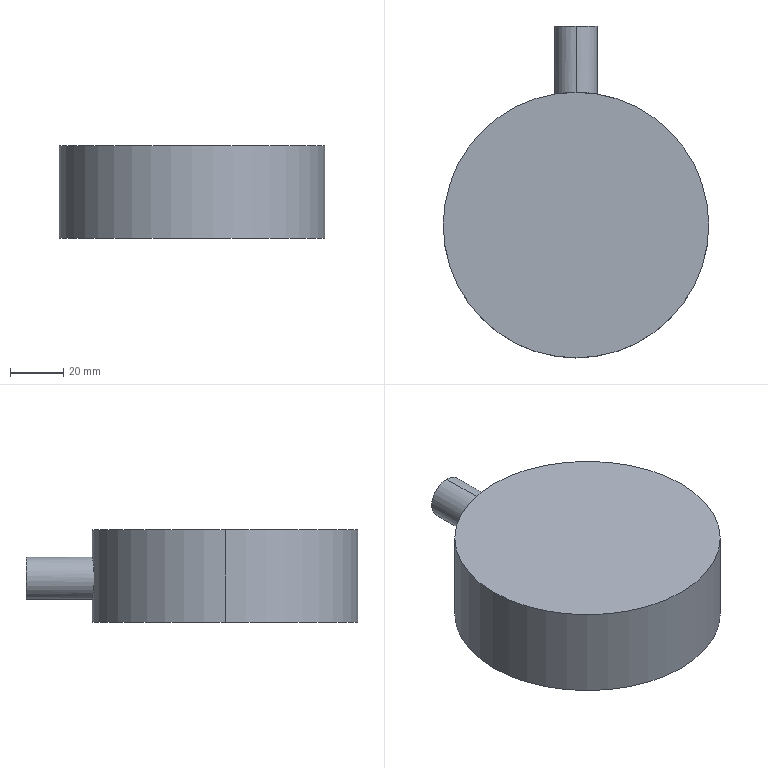Part | SolidWorks | features Extrusion 1, ICE 1 | 1 solid | 7 faces | box 100 x 125 x 35 mm | volume 279948 mm3 | cylinder 4 | plane 3 | commonest cylinder face diameters 16 x2 100 x2
STEP:
#1=CARTESIAN_POINT('',(0.,75.,24.624));
#2=VERTEX_POINT('',#1);
#3=CARTESIAN_POINT('',(0.,75.,8.624));
#4=VERTEX_POINT('',#3);
#5=CARTESIAN_POINT('',(0.,75.,16.624));
#6=DIRECTION('',(0.,1.,0.));
#7=DIRECTION('',(0.,0.,1.));
#8=AXIS2_PLACEMENT_3D('',#5,#6,#7);
#9=CIRCLE('',#8,8.);
#10=EDGE_CURVE('',#2,#4,#9,.T.);
#11=ORIENTED_EDGE('',*,*,#10,.F.);
#12=CARTESIAN_POINT('',(0.,50.,24.624));
#13=VERTEX_POINT('',#12);
#14=CARTESIAN_POINT('',(0.,75.,24.624));
#15=DIRECTION('',(0.,-1.,0.));
#16=VECTOR('',#15,1000.);
#17=LINE('',#14,#16);
#18=EDGE_CURVE('',#2,#13,#17,.T.);
#19=ORIENTED_EDGE('',*,*,#18,.T.);
#20=CARTESIAN_POINT('',(0.,50.,8.624));
#21=VERTEX_POINT('',#20);
#22=CARTESIAN_POINT('',(0.,50.,24.624));
#23=CARTESIAN_POINT('',(0.5224,50.,24.624));
#24=CARTESIAN_POINT('',(1.042,49.992,24.574));
#25=CARTESIAN_POINT('',(1.818,49.968,24.419));
#26=CARTESIAN_POINT('',(2.075,49.958,24.355));
#27=CARTESIAN_POINT('',(2.576,49.934,24.203));
#28=CARTESIAN_POINT('',(3.067,49.908,24.027));
#29=CARTESIAN_POINT('',(3.538,49.875,23.804));
#30=CARTESIAN_POINT('',(4.,49.84,23.557));
#31=CARTESIAN_POINT('',(4.228,49.821,23.421));
#32=CARTESIAN_POINT('',(4.882,49.763,22.984));
#33=CARTESIAN_POINT('',(5.284,49.721,22.653));
#34=CARTESIAN_POINT('',(6.022,49.637,21.916));
#35=CARTESIAN_POINT('',(6.36,49.595,21.505));
#36=CARTESIAN_POINT('',(6.94,49.517,20.638));
#37=CARTESIAN_POINT('',(7.186,49.481,20.179));
#38=CARTESIAN_POINT('',(7.488,49.436,19.452));
#39=CARTESIAN_POINT('',(7.578,49.423,19.203));
#40=CARTESIAN_POINT('',(7.73,49.399,18.701));
#41=CARTESIAN_POINT('',(7.794,49.389,18.447));
#42=CARTESIAN_POINT('',(7.947,49.364,17.68));
#43=CARTESIAN_POINT('',(8.,49.356,17.158));
#44=CARTESIAN_POINT('',(8.,49.356,16.101));
#45=CARTESIAN_POINT('',(7.949,49.364,15.581));
#46=CARTESIAN_POINT('',(7.797,49.388,14.813));
#47=CARTESIAN_POINT('',(7.733,49.398,14.559));
#48=CARTESIAN_POINT('',(7.581,49.422,14.055));
#49=CARTESIAN_POINT('',(7.491,49.436,13.805));
#50=CARTESIAN_POINT('',(7.191,49.481,13.08));
#51=CARTESIAN_POINT('',(6.946,49.516,12.62));
#52=CARTESIAN_POINT('',(6.51,49.575,11.968));
#53=CARTESIAN_POINT('',(6.353,49.595,11.755));
#54=CARTESIAN_POINT('',(6.02,49.637,11.349));
#55=CARTESIAN_POINT('',(5.845,49.658,11.155));
#56=CARTESIAN_POINT('',(5.293,49.72,10.603));
#57=CARTESIAN_POINT('',(4.891,49.762,10.272));
#58=CARTESIAN_POINT('',(4.016,49.84,9.685));
#59=CARTESIAN_POINT('',(3.553,49.876,9.438));
#60=CARTESIAN_POINT('',(2.832,49.92,9.138));
#61=CARTESIAN_POINT('',(2.586,49.934,9.049));
#62=CARTESIAN_POINT('',(2.085,49.957,8.896));
#63=CARTESIAN_POINT('',(1.827,49.967,8.831));
#64=CARTESIAN_POINT('',(1.052,49.992,8.676));
#65=CARTESIAN_POINT('',(0.5294,50.,8.624));
#66=CARTESIAN_POINT('',(0.,50.,8.624));
#67=B_SPLINE_CURVE_WITH_KNOTS('',3,(#22,#23,#24,#25,#26,#27,#28,#29,#30,#31,#32,#33,#34,#35,#36,#37,#38,#39,#40,#41,#42,#43,#44,#45,#46,#47,#48,#49,#50,#51,#52,#53,#54,#55,#56,#57,#58,#59,#60,#61,#62,#63,#64,#65,#66),.UNSPECIFIED.,.F.,.F.,(4,2,2,1,2,2,2,2,2,2,2,2,2,2,2,2,2,2,2,2,2,2,4),(0.02505,0.02662,0.0274,0.02818,0.02897,0.02975,0.03131,0.03288,0.03444,0.03523,0.03601,0.03757,0.03914,0.03992,0.04071,0.04227,0.04305,0.04384,0.0454,0.04697,0.04775,0.04853,0.0501),.UNSPECIFIED.);
#68=EDGE_CURVE('',#13,#21,#67,.T.);
#69=ORIENTED_EDGE('',*,*,#68,.T.);
#70=CARTESIAN_POINT('',(0.,75.,8.624));
#71=DIRECTION('',(0.,-1.,0.));
#72=VECTOR('',#71,1000.);
#73=LINE('',#70,#72);
#74=EDGE_CURVE('',#4,#21,#73,.T.);
#75=ORIENTED_EDGE('',*,*,#74,.F.);
#76=EDGE_LOOP('',(#11,#19,#69,#75));
#77=FACE_OUTER_BOUND('',#76,.T.);
#78=CARTESIAN_POINT('',(0.,75.,16.624));
#79=DIRECTION('',(0.,-1.,0.));
#80=DIRECTION('',(0.,0.,-1.));
#81=AXIS2_PLACEMENT_3D('',#78,#79,#80);
#82=CYLINDRICAL_SURFACE('',#81,8.);
#83=ADVANCED_FACE('',(#77),#82,.T.);
#84=CARTESIAN_POINT('',(0.,50.,8.624));
#85=CARTESIAN_POINT('',(-0.5295,50.,8.624));
#86=CARTESIAN_POINT('',(-1.05,49.992,8.676));
#87=CARTESIAN_POINT('',(-1.818,49.968,8.829));
#88=CARTESIAN_POINT('',(-2.072,49.958,8.893));
#89=CARTESIAN_POINT('',(-2.575,49.934,9.045));
#90=CARTESIAN_POINT('',(-2.824,49.921,9.135));
#91=CARTESIAN_POINT('',(-3.551,49.876,9.436));
#92=CARTESIAN_POINT('',(-4.01,49.841,9.682));
#93=CARTESIAN_POINT('',(-4.662,49.783,10.118));
#94=CARTESIAN_POINT('',(-4.874,49.762,10.275));
#95=CARTESIAN_POINT('',(-5.28,49.721,10.609));
#96=CARTESIAN_POINT('',(-5.474,49.7,10.785));
#97=CARTESIAN_POINT('',(-6.026,49.637,11.337));
#98=CARTESIAN_POINT('',(-6.357,49.595,11.739));
#99=CARTESIAN_POINT('',(-6.796,49.536,12.395));
#100=CARTESIAN_POINT('',(-6.932,49.517,12.622));
#101=CARTESIAN_POINT('',(-7.178,49.482,13.083));
#102=CARTESIAN_POINT('',(-7.401,49.449,13.554));
#103=CARTESIAN_POINT('',(-7.578,49.423,14.046));
#104=CARTESIAN_POINT('',(-7.73,49.399,14.547));
#105=CARTESIAN_POINT('',(-7.795,49.389,14.804));
#106=CARTESIAN_POINT('',(-7.949,49.364,15.579));
#107=CARTESIAN_POINT('',(-8.,49.356,16.099));
#108=CARTESIAN_POINT('',(-8.,49.356,17.144));
#109=CARTESIAN_POINT('',(-7.948,49.364,17.675));
#110=CARTESIAN_POINT('',(-7.743,49.397,18.702));
#111=CARTESIAN_POINT('',(-7.592,49.421,19.201));
#112=CARTESIAN_POINT('',(-7.291,49.466,19.928));
#113=CARTESIAN_POINT('',(-7.177,49.482,20.168));
#114=CARTESIAN_POINT('',(-6.93,49.518,20.63));
#115=CARTESIAN_POINT('',(-6.795,49.536,20.854));
#116=CARTESIAN_POINT('',(-6.361,49.595,21.504));
#117=CARTESIAN_POINT('',(-6.03,49.637,21.908));
#118=CARTESIAN_POINT('',(-5.284,49.721,22.654));
#119=CARTESIAN_POINT('',(-4.881,49.763,22.984));
#120=CARTESIAN_POINT('',(-4.232,49.821,23.418));
#121=CARTESIAN_POINT('',(-4.008,49.84,23.553));
#122=CARTESIAN_POINT('',(-3.545,49.875,23.801));
#123=CARTESIAN_POINT('',(-3.305,49.891,23.914));
#124=CARTESIAN_POINT('',(-2.579,49.936,24.215));
#125=CARTESIAN_POINT('',(-2.08,49.959,24.367));
#126=CARTESIAN_POINT('',(-1.31,49.983,24.521));
#127=CARTESIAN_POINT('',(-1.048,49.99,24.56));
#128=CARTESIAN_POINT('',(-0.5232,49.998,24.612));
#129=CARTESIAN_POINT('',(-0.2613,50.,24.624));
#130=CARTESIAN_POINT('',(0.,50.,24.624));
#131=B_SPLINE_CURVE_WITH_KNOTS('',3,(#84,#85,#86,#87,#88,#89,#90,#91,#92,#93,#94,#95,#96,#97,#98,#99,#100,#101,#102,#103,#104,#105,#106,#107,#108,#109,#110,#111,#112,#113,#114,#115,#116,#117,#118,#119,#120,#121,#122,#123,#124,#125,#126,#127,#128,#129,#130),.UNSPECIFIED.,.F.,.F.,(4,2,2,2,2,2,2,2,2,1,2,2,2,2,2,2,2,2,2,2,2,2,2,4),(0.,0.001566,0.002349,0.003131,0.004697,0.00548,0.006263,0.007829,0.008612,0.009394,0.01018,0.01096,0.01253,0.01409,0.01566,0.01644,0.01722,0.01879,0.02035,0.02114,0.02192,0.02349,0.02427,0.02505),.UNSPECIFIED.);
#132=EDGE_CURVE('',#21,#13,#131,.T.);
#133=ORIENTED_EDGE('',*,*,#132,.F.);
#134=ORIENTED_EDGE('',*,*,#68,.F.);
#135=EDGE_LOOP('',(#133,#134));
#136=FACE_BOUND('',#135,.T.);
#137=CARTESIAN_POINT('',(50.,0.,35.));
#138=VERTEX_POINT('',#137);
#139=CARTESIAN_POINT('',(-50.,0.,35.));
#140=VERTEX_POINT('',#139);
#141=CARTESIAN_POINT('',(0.,0.,35.));
#142=DIRECTION('',(0.,0.,1.));
#143=DIRECTION('',(1.,0.,0.));
#144=AXIS2_PLACEMENT_3D('',#141,#142,#143);
#145=CIRCLE('',#144,50.);
#146=EDGE_CURVE('',#138,#140,#145,.T.);
#147=ORIENTED_EDGE('',*,*,#146,.F.);
#148=CARTESIAN_POINT('',(50.,0.,0.));
#149=VERTEX_POINT('',#148);
#150=CARTESIAN_POINT('',(50.,0.,35.));
#151=DIRECTION('',(0.,0.,-1.));
#152=VECTOR('',#151,1000.);
#153=LINE('',#150,#152);
#154=EDGE_CURVE('',#138,#149,#153,.T.);
#155=ORIENTED_EDGE('',*,*,#154,.T.);
#156=CARTESIAN_POINT('',(-50.,0.,0.));
#157=VERTEX_POINT('',#156);
#158=CARTESIAN_POINT('',(0.,0.,0.));
#159=DIRECTION('',(0.,0.,1.));
#160=DIRECTION('',(1.,0.,0.));
#161=AXIS2_PLACEMENT_3D('',#158,#159,#160);
#162=CIRCLE('',#161,50.);
#163=EDGE_CURVE('',#149,#157,#162,.T.);
#164=ORIENTED_EDGE('',*,*,#163,.T.);
#165=CARTESIAN_POINT('',(-50.,0.,35.));
#166=DIRECTION('',(0.,0.,-1.));
#167=VECTOR('',#166,1000.);
#168=LINE('',#165,#167);
#169=EDGE_CURVE('',#140,#157,#168,.T.);
#170=ORIENTED_EDGE('',*,*,#169,.F.);
#171=EDGE_LOOP('',(#147,#155,#164,#170));
#172=FACE_OUTER_BOUND('',#171,.T.);
#173=CARTESIAN_POINT('',(0.,0.,35.));
#174=DIRECTION('',(0.,0.,-1.));
#175=DIRECTION('',(-1.,0.,0.));
#176=AXIS2_PLACEMENT_3D('',#173,#174,#175);
#177=CYLINDRICAL_SURFACE('',#176,50.);
#178=ADVANCED_FACE('',(#136,#172),#177,.T.);
#179=ORIENTED_EDGE('',*,*,#154,.F.);
#180=CARTESIAN_POINT('',(0.,0.,35.));
#181=DIRECTION('',(0.,0.,1.));
#182=DIRECTION('',(1.,0.,0.));
#183=AXIS2_PLACEMENT_3D('',#180,#181,#182);
#184=CIRCLE('',#183,50.);
#185=EDGE_CURVE('',#140,#138,#184,.T.);
#186=ORIENTED_EDGE('',*,*,#185,.F.);
#187=ORIENTED_EDGE('',*,*,#169,.T.);
#188=CARTESIAN_POINT('',(0.,0.,0.));
#189=DIRECTION('',(0.,0.,1.));
#190=DIRECTION('',(1.,0.,0.));
#191=AXIS2_PLACEMENT_3D('',#188,#189,#190);
#192=CIRCLE('',#191,50.);
#193=EDGE_CURVE('',#157,#149,#192,.T.);
#194=ORIENTED_EDGE('',*,*,#193,.T.);
#195=EDGE_LOOP('',(#179,#186,#187,#194));
#196=FACE_OUTER_BOUND('',#195,.T.);
#197=CARTESIAN_POINT('',(0.,0.,35.));
#198=DIRECTION('',(0.,0.,-1.));
#199=DIRECTION('',(-1.,0.,0.));
#200=AXIS2_PLACEMENT_3D('',#197,#198,#199);
#201=CYLINDRICAL_SURFACE('',#200,50.);
#202=ADVANCED_FACE('',(#196),#201,.T.);
#203=ORIENTED_EDGE('',*,*,#185,.T.);
#204=ORIENTED_EDGE('',*,*,#146,.T.);
#205=EDGE_LOOP('',(#203,#204));
#206=FACE_OUTER_BOUND('',#205,.T.);
#207=CARTESIAN_POINT('',(0.,0.,35.));
#208=DIRECTION('',(0.,0.,1.));
#209=DIRECTION('',(1.,0.,0.));
#210=AXIS2_PLACEMENT_3D('',#207,#208,#209);
#211=PLANE('',#210);
#212=ADVANCED_FACE('',(#206),#211,.T.);
#213=ORIENTED_EDGE('',*,*,#193,.F.);
#214=ORIENTED_EDGE('',*,*,#163,.F.);
#215=EDGE_LOOP('',(#213,#214));
#216=FACE_OUTER_BOUND('',#215,.T.);
#217=CARTESIAN_POINT('',(0.,0.,0.));
#218=DIRECTION('',(0.,0.,1.));
#219=DIRECTION('',(1.,0.,0.));
#220=AXIS2_PLACEMENT_3D('',#217,#218,#219);
#221=PLANE('',#220);
#222=ADVANCED_FACE('',(#216),#221,.F.);
#223=ORIENTED_EDGE('',*,*,#18,.F.);
#224=CARTESIAN_POINT('',(0.,75.,16.624));
#225=DIRECTION('',(0.,1.,0.));
#226=DIRECTION('',(0.,0.,1.));
#227=AXIS2_PLACEMENT_3D('',#224,#225,#226);
#228=CIRCLE('',#227,8.);
#229=EDGE_CURVE('',#4,#2,#228,.T.);
#230=ORIENTED_EDGE('',*,*,#229,.F.);
#231=ORIENTED_EDGE('',*,*,#74,.T.);
#232=ORIENTED_EDGE('',*,*,#132,.T.);
#233=EDGE_LOOP('',(#223,#230,#231,#232));
#234=FACE_OUTER_BOUND('',#233,.T.);
#235=CARTESIAN_POINT('',(0.,75.,16.624));
#236=DIRECTION('',(0.,-1.,0.));
#237=DIRECTION('',(0.,0.,-1.));
#238=AXIS2_PLACEMENT_3D('',#235,#236,#237);
#239=CYLINDRICAL_SURFACE('',#238,8.);
#240=ADVANCED_FACE('',(#234),#239,.T.);
#241=ORIENTED_EDGE('',*,*,#229,.T.);
#242=ORIENTED_EDGE('',*,*,#10,.T.);
#243=EDGE_LOOP('',(#241,#242));
#244=FACE_OUTER_BOUND('',#243,.T.);
#245=CARTESIAN_POINT('',(0.,75.,16.624));
#246=DIRECTION('',(0.,1.,0.));
#247=DIRECTION('',(0.,0.,1.));
#248=AXIS2_PLACEMENT_3D('',#245,#246,#247);
#249=PLANE('',#248);
#250=ADVANCED_FACE('',(#244),#249,.T.);
#251=CLOSED_SHELL('',(#83,#178,#202,#212,#222,#240,#250));
#252=MANIFOLD_SOLID_BREP('',#251);
#253=CARTESIAN_POINT('',(0.,0.,0.));
#254=DIRECTION('',(0.,0.,1.));
#255=DIRECTION('',(1.,0.,0.));
#256=AXIS2_PLACEMENT_3D('',#253,#254,#255);
#257=(LENGTH_UNIT()NAMED_UNIT(*)SI_UNIT(.MILLI.,.METRE.));
#258=UNCERTAINTY_MEASURE_WITH_UNIT(LENGTH_MEASURE(0.00001),#257,'','');
#259=(NAMED_UNIT(*)PLANE_ANGLE_UNIT()SI_UNIT($,.RADIAN.));
#260=(NAMED_UNIT(*)SI_UNIT($,.STERADIAN.)SOLID_ANGLE_UNIT());
#261=(GEOMETRIC_REPRESENTATION_CONTEXT(3)GLOBAL_UNCERTAINTY_ASSIGNED_CONTEXT((#258))GLOBAL_UNIT_ASSIGNED_CONTEXT((#257,#259,#260))REPRESENTATION_CONTEXT('',''));
#262=ADVANCED_BREP_SHAPE_REPRESENTATION('',(#252,#256),#261);